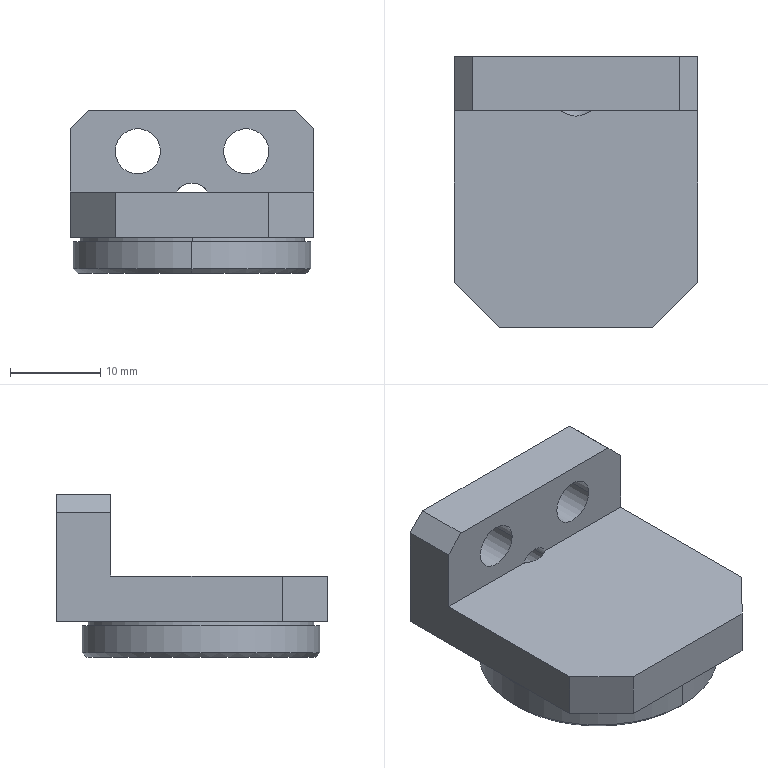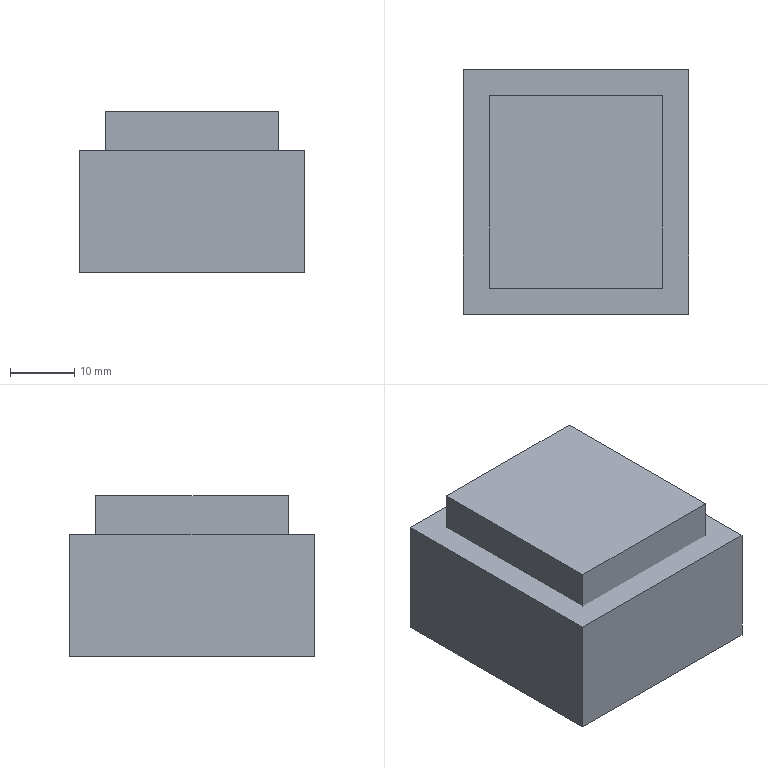CAM job | NX | 3+2 milling, drilling | part box 27 x 30 x 18 mm | stock box 35 x 38 x 25 mm
Tools:
number,name,description,diameter,corner_radius,flute_length,length,flutes
11,D10JING,Milling Tool-5 Parameters,10.0,0.0,50.0,75.0,2
10,D10,Milling Tool-5 Parameters,10.0,0.0,50.0,75.0,2
5,D4R0.5,Milling Tool-5 Parameters,4.0,0.5,50.0,75.0,2
7,D6A45,Milling Tool-5 Parameters,6.0,0.0,50.0,75.0,2
15,5.0ZT,Drilling Tool,5.0,0.0,35.0,50.0,2
3,D3,Milling Tool-5 Parameters,3.0,0.0,50.0,75.0,2
8,T8H0.5,Milling Tool-T Cutter,8.0,,0.5,30.0,4
14,D2.4XYD,Thread Mill,2.4,0.0,0.635,80.0,2
Operations:
program,operation,operation_type,tool,method,geometry_group,spindle_rpm,surface_speed,feed_per_tooth,feed_cut,feed_plunge,cut_length_mm,path_length_mm,cut_time_min,machine_time_min
1,FLOOR_WALL,VolumeBased25DMillingOperation,D10JING,METHOD,A,9500.0,298.0,0.0658,1250.0,100.0,426.997,480.997,0.3416,0.347
1,ZLEVEL_PROFILE,ZLevelMilling,D10,METHOD,A,9500.0,298.0,0.1579,3000.0,1000.0,5115.212,5190.212,1.73,1.738
1,FLOOR_WALL_1,VolumeBased25DMillingOperation,D10,METHOD,A,9500.0,179.0,0.1316,2500.0,1000.0,2467.376,2751.433,1.068,1.097
1,ZLEVEL_PROFILE_COPY_1,ZLevelMilling,D10JING,METHOD,A,9500.0,298.0,0.0632,1200.0,1000.0,147.897,240.897,0.1239,0.1332
1,FLOOR_WALL_1_1,VolumeBased25DMillingOperation,D10JING,METHOD,A,9500.0,298.0,0.0658,1250.0,100.0,278.014,370.714,0.2224,0.2317
1,ZLEVEL_PROFILE_1,ZLevelMilling,D4R0.5,METHOD,A,9500.0,119.0,0.1579,3000.0,1000.0,586.91,739.839,0.1983,0.2136
1,PLANAR_MILL_COPY,PlanarMilling,D6A45,METHOD,A,9500.0,179.0,0.0658,1250.0,100.0,77.394,136.394,0.0619,0.0678
1,PLANAR_MILL_COPY_COPY,PlanarMilling,D6A45,METHOD,A,9500.0,179.0,0.0658,1250.0,100.0,71.168,148.168,0.0569,0.0646
2,FLOOR_WALL_COPY,VolumeBased25DMillingOperation,D10JING,METHOD,B,9500.0,298.0,0.0658,1250.0,100.0,3849.958,4813.923,3.08,3.176
2,ZLEVEL_PROFILE_COPY,ZLevelMilling,D10,METHOD,B,9500.0,298.0,0.1579,3000.0,1000.0,985.483,1046.483,0.354,0.3601
2,ZLEVEL_PROFILE_COPY_1_COPY,ZLevelMilling,D10JING,METHOD,B,9500.0,298.0,0.0632,1200.0,1000.0,122.403,187.403,0.1027,0.1092
2,PLANAR_MILL_COPY_COPY_1,PlanarMilling,D6A45,METHOD,B,9500.0,179.0,0.0658,1250.0,100.0,92.325,151.325,0.0739,0.0798
2,PLANAR_MILL,PlanarMilling,T8H0.5,METHOD,B,5000.0,125.0,0.05,1000.0,100.0,1699.921,1761.921,1.7,1.706
2,BOSS_THREAD_MILLING,ThreadMilling,D2.4XYD,METHOD,B,5000.0,37.0,0.1,1000.0,100.0,5522.499,5625.706,5.522,5.533
3,DRILLING,Operation,D6A45,METHOD,C,5000.0,94.0,0.025,250.0,0.0,12.0,111.044,0.048,0.0579
3,DRILLING_COPY,Operation,5.0ZT,METHOD,C,5000.0,94.0,0.025,250.0,0.0,24.004,123.378,0.096,0.106
3,ZLEVEL_PROFILE_COPY_COPY_1,ZLevelMilling,D3,METHOD,C,9500.0,89.0,0.0632,1200.0,1000.0,99.987,163.954,0.0871,0.0935
3,PLANAR_MILL_COPY_COPY_1_COPY,PlanarMilling,D6A45,METHOD,C,9500.0,179.0,0.0658,1250.0,100.0,131.45,394.406,0.1052,0.1315
3,刀补3,ZLevelMilling,D3,METHOD,C,9500.0,89.0,0.0632,1200.0,1000.0,14.169,78.431,0.012,0.0185